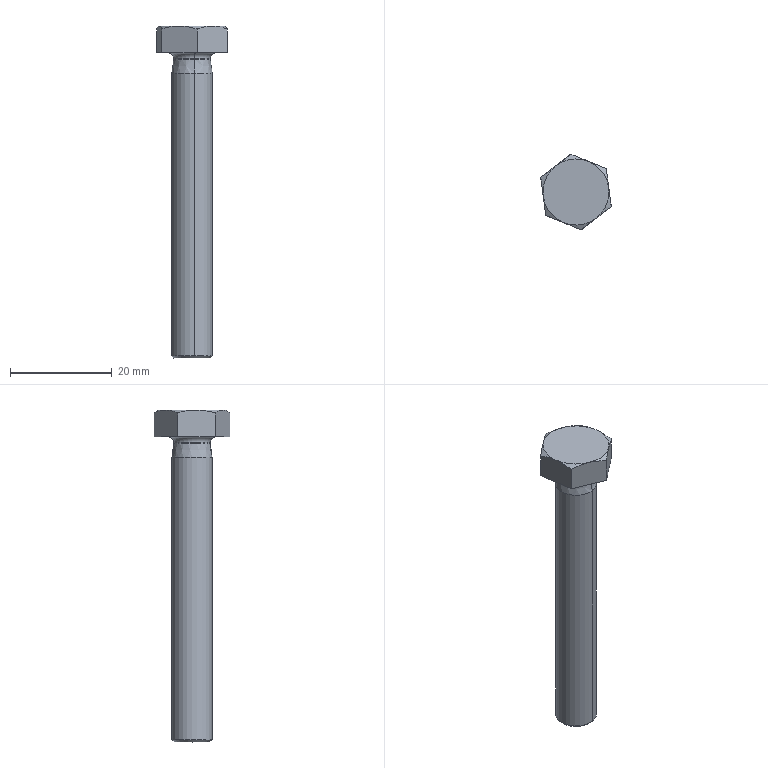Part | STEP file | Chamfer 1-4 | 1 solid | 25 faces | box 13.89 x 14.875 x 65.3 mm | volume 3768 mm3 | cone 10 | plane 9 | torus 4 | cylinder 2 | commonest cylinder face diameters 8 x2
STEP:
#1=CARTESIAN_POINT('',(-881.108,35.613,3046.7));
#2=VERTEX_POINT('',#1);
#3=CARTESIAN_POINT('',(-881.256,36.703,3045.6));
#4=VERTEX_POINT('',#3);
#5=CARTESIAN_POINT('',(-881.108,35.613,3045.6));
#6=DIRECTION('',(-0.991,-0.1342,-0.000000001));
#7=DIRECTION('',(-0.000000001,0.,1.));
#8=AXIS2_PLACEMENT_3D('',#5,#6,#7);
#9=CIRCLE('',#8,1.1);
#10=EDGE_CURVE('',#2,#4,#9,.T.);
#11=ORIENTED_EDGE('',*,*,#10,.T.);
#12=CARTESIAN_POINT('',(-882.221,43.826,3045.6));
#13=VERTEX_POINT('',#12);
#14=CARTESIAN_POINT('',(-881.738,40.264,3045.6));
#15=DIRECTION('',(-0.000000001,0.,1.));
#16=DIRECTION('',(0.1342,-0.991,0.));
#17=AXIS2_PLACEMENT_3D('',#14,#15,#16);
#18=CIRCLE('',#17,3.594);
#19=EDGE_CURVE('',#4,#13,#18,.T.);
#20=ORIENTED_EDGE('',*,*,#19,.T.);
#21=CARTESIAN_POINT('',(-882.368,44.916,3046.7));
#22=VERTEX_POINT('',#21);
#23=CARTESIAN_POINT('',(-882.368,44.916,3045.6));
#24=DIRECTION('',(0.991,0.1342,0.000000001));
#25=DIRECTION('',(0.1342,-0.991,0.));
#26=AXIS2_PLACEMENT_3D('',#23,#24,#25);
#27=CIRCLE('',#26,1.1);
#28=EDGE_CURVE('',#22,#13,#27,.T.);
#29=ORIENTED_EDGE('',*,*,#28,.F.);
#30=CARTESIAN_POINT('',(-881.738,40.264,3046.7));
#31=DIRECTION('',(-0.000000001,0.,1.));
#32=DIRECTION('',(0.1342,-0.991,0.));
#33=AXIS2_PLACEMENT_3D('',#30,#31,#32);
#34=CIRCLE('',#33,4.694);
#35=EDGE_CURVE('',#2,#22,#34,.T.);
#36=ORIENTED_EDGE('',*,*,#35,.F.);
#37=EDGE_LOOP('',(#11,#20,#29,#36));
#38=FACE_OUTER_BOUND('',#37,.T.);
#39=CARTESIAN_POINT('',(-881.738,40.264,3045.6));
#40=DIRECTION('',(-0.000000001,0.,1.));
#41=DIRECTION('',(-0.1342,0.991,0.));
#42=AXIS2_PLACEMENT_3D('',#39,#40,#41);
#43=TOROIDAL_SURFACE('',#42,4.694,1.1);
#44=ADVANCED_FACE('',(#38),#43,.F.);
#45=ORIENTED_EDGE('',*,*,#28,.T.);
#46=CARTESIAN_POINT('',(-881.738,40.264,3045.6));
#47=DIRECTION('',(-0.000000001,0.,1.));
#48=DIRECTION('',(0.1342,-0.991,0.));
#49=AXIS2_PLACEMENT_3D('',#46,#47,#48);
#50=CIRCLE('',#49,3.594);
#51=EDGE_CURVE('',#13,#4,#50,.T.);
#52=ORIENTED_EDGE('',*,*,#51,.T.);
#53=ORIENTED_EDGE('',*,*,#10,.F.);
#54=CARTESIAN_POINT('',(-881.738,40.264,3046.7));
#55=DIRECTION('',(-0.000000001,0.,1.));
#56=DIRECTION('',(0.1342,-0.991,0.));
#57=AXIS2_PLACEMENT_3D('',#54,#55,#56);
#58=CIRCLE('',#57,4.694);
#59=EDGE_CURVE('',#22,#2,#58,.T.);
#60=ORIENTED_EDGE('',*,*,#59,.F.);
#61=EDGE_LOOP('',(#45,#52,#53,#60));
#62=FACE_OUTER_BOUND('',#61,.T.);
#63=CARTESIAN_POINT('',(-881.738,40.264,3045.6));
#64=DIRECTION('',(-0.000000001,0.,1.));
#65=DIRECTION('',(-0.1342,0.991,0.));
#66=AXIS2_PLACEMENT_3D('',#63,#64,#65);
#67=TOROIDAL_SURFACE('',#66,4.694,1.1);
#68=ADVANCED_FACE('',(#62),#67,.F.);
#69=CARTESIAN_POINT('',(-882.215,43.788,2986.7));
#70=VERTEX_POINT('',#69);
#71=CARTESIAN_POINT('',(-881.261,36.741,2986.7));
#72=VERTEX_POINT('',#71);
#73=CARTESIAN_POINT('',(-881.738,40.264,2986.7));
#74=DIRECTION('',(0.000000001,0.,-1.));
#75=DIRECTION('',(0.1342,-0.991,0.));
#76=AXIS2_PLACEMENT_3D('',#73,#74,#75);
#77=CIRCLE('',#76,3.556);
#78=EDGE_CURVE('',#70,#72,#77,.T.);
#79=ORIENTED_EDGE('',*,*,#78,.F.);
#80=CARTESIAN_POINT('',(-882.275,44.228,2987.144));
#81=VERTEX_POINT('',#80);
#82=CARTESIAN_POINT('',(-882.275,44.228,2987.144));
#83=DIRECTION('',(0.09489,-0.7007,-0.7071));
#84=VECTOR('',#83,1000.);
#85=LINE('',#82,#84);
#86=EDGE_CURVE('',#81,#70,#85,.T.);
#87=ORIENTED_EDGE('',*,*,#86,.F.);
#88=CARTESIAN_POINT('',(-881.202,36.3,2987.144));
#89=VERTEX_POINT('',#88);
#90=CARTESIAN_POINT('',(-881.738,40.264,2987.144));
#91=DIRECTION('',(-0.000000001,0.,1.));
#92=DIRECTION('',(0.1342,-0.991,0.));
#93=AXIS2_PLACEMENT_3D('',#90,#91,#92);
#94=CIRCLE('',#93,4.);
#95=EDGE_CURVE('',#89,#81,#94,.T.);
#96=ORIENTED_EDGE('',*,*,#95,.F.);
#97=CARTESIAN_POINT('',(-881.202,36.3,2987.144));
#98=DIRECTION('',(-0.09489,0.7007,-0.7071));
#99=VECTOR('',#98,1000.);
#100=LINE('',#97,#99);
#101=EDGE_CURVE('',#89,#72,#100,.T.);
#102=ORIENTED_EDGE('',*,*,#101,.T.);
#103=EDGE_LOOP('',(#79,#87,#96,#102));
#104=FACE_OUTER_BOUND('',#103,.T.);
#105=CARTESIAN_POINT('',(-881.738,40.264,2987.144));
#106=DIRECTION('',(-0.000000001,0.,1.));
#107=DIRECTION('',(-0.1342,0.991,0.));
#108=AXIS2_PLACEMENT_3D('',#105,#106,#107);
#109=CONICAL_SURFACE('',#108,4.,0.7854);
#110=ADVANCED_FACE('',(#104),#109,.T.);
#111=ORIENTED_EDGE('',*,*,#51,.F.);
#112=CARTESIAN_POINT('',(-882.222,43.837,3045.443));
#113=VERTEX_POINT('',#112);
#114=CARTESIAN_POINT('',(-882.368,44.916,3045.6));
#115=DIRECTION('',(-0.991,-0.1342,-0.000000001));
#116=DIRECTION('',(0.1342,-0.991,0.));
#117=AXIS2_PLACEMENT_3D('',#114,#115,#116);
#118=CIRCLE('',#117,1.1);
#119=EDGE_CURVE('',#113,#13,#118,.T.);
#120=ORIENTED_EDGE('',*,*,#119,.F.);
#121=CARTESIAN_POINT('',(-881.254,36.692,3045.443));
#122=VERTEX_POINT('',#121);
#123=CARTESIAN_POINT('',(-881.738,40.264,3045.443));
#124=DIRECTION('',(-0.000000001,0.,1.));
#125=DIRECTION('',(0.1342,-0.991,0.));
#126=AXIS2_PLACEMENT_3D('',#123,#124,#125);
#127=CIRCLE('',#126,3.605);
#128=EDGE_CURVE('',#113,#122,#127,.T.);
#129=ORIENTED_EDGE('',*,*,#128,.T.);
#130=CARTESIAN_POINT('',(-881.108,35.613,3045.6));
#131=DIRECTION('',(0.991,0.1342,0.000000001));
#132=DIRECTION('',(-0.000000001,0.,1.));
#133=AXIS2_PLACEMENT_3D('',#130,#131,#132);
#134=CIRCLE('',#133,1.1);
#135=EDGE_CURVE('',#122,#4,#134,.T.);
#136=ORIENTED_EDGE('',*,*,#135,.T.);
#137=EDGE_LOOP('',(#111,#120,#129,#136));
#138=FACE_OUTER_BOUND('',#137,.T.);
#139=CARTESIAN_POINT('',(-881.738,40.264,3045.6));
#140=DIRECTION('',(-0.000000001,0.,1.));
#141=DIRECTION('',(-0.1342,0.991,0.));
#142=AXIS2_PLACEMENT_3D('',#139,#140,#141);
#143=TOROIDAL_SURFACE('',#142,4.694,1.1);
#144=ADVANCED_FACE('',(#138),#143,.F.);
#145=ORIENTED_EDGE('',*,*,#95,.T.);
#146=CARTESIAN_POINT('',(-882.275,44.228,3042.7));
#147=VERTEX_POINT('',#146);
#148=CARTESIAN_POINT('',(-882.275,44.228,3046.7));
#149=DIRECTION('',(0.000000001,0.,-1.));
#150=VECTOR('',#149,1000.);
#151=LINE('',#148,#150);
#152=EDGE_CURVE('',#147,#81,#151,.T.);
#153=ORIENTED_EDGE('',*,*,#152,.F.);
#154=CARTESIAN_POINT('',(-881.202,36.3,3042.7));
#155=VERTEX_POINT('',#154);
#156=CARTESIAN_POINT('',(-881.738,40.264,3042.7));
#157=DIRECTION('',(-0.000000001,0.,1.));
#158=DIRECTION('',(0.1342,-0.991,0.));
#159=AXIS2_PLACEMENT_3D('',#156,#157,#158);
#160=CIRCLE('',#159,4.);
#161=EDGE_CURVE('',#155,#147,#160,.T.);
#162=ORIENTED_EDGE('',*,*,#161,.F.);
#163=CARTESIAN_POINT('',(-881.202,36.3,3046.7));
#164=DIRECTION('',(0.000000001,0.,-1.));
#165=VECTOR('',#164,1000.);
#166=LINE('',#163,#165);
#167=EDGE_CURVE('',#155,#89,#166,.T.);
#168=ORIENTED_EDGE('',*,*,#167,.T.);
#169=EDGE_LOOP('',(#145,#153,#162,#168));
#170=FACE_OUTER_BOUND('',#169,.T.);
#171=CARTESIAN_POINT('',(-881.738,40.264,3046.7));
#172=DIRECTION('',(-0.000000001,0.,1.));
#173=DIRECTION('',(-0.1342,0.991,0.));
#174=AXIS2_PLACEMENT_3D('',#171,#172,#173);
#175=CYLINDRICAL_SURFACE('',#174,4.);
#176=ADVANCED_FACE('',(#170),#175,.T.);
#177=CARTESIAN_POINT('',(-881.738,40.264,3045.443));
#178=DIRECTION('',(-0.000000001,0.,1.));
#179=DIRECTION('',(0.1342,-0.991,0.));
#180=AXIS2_PLACEMENT_3D('',#177,#178,#179);
#181=CIRCLE('',#180,3.605);
#182=EDGE_CURVE('',#122,#113,#181,.T.);
#183=ORIENTED_EDGE('',*,*,#182,.F.);
#184=CARTESIAN_POINT('',(-881.202,36.3,3042.7));
#185=DIRECTION('',(0.01911,-0.1411,-0.9898));
#186=VECTOR('',#185,1000.);
#187=LINE('',#184,#186);
#188=EDGE_CURVE('',#122,#155,#187,.T.);
#189=ORIENTED_EDGE('',*,*,#188,.T.);
#190=ORIENTED_EDGE('',*,*,#161,.T.);
#191=CARTESIAN_POINT('',(-882.275,44.228,3042.7));
#192=DIRECTION('',(-0.01911,0.1411,-0.9898));
#193=VECTOR('',#192,1000.);
#194=LINE('',#191,#193);
#195=EDGE_CURVE('',#113,#147,#194,.T.);
#196=ORIENTED_EDGE('',*,*,#195,.F.);
#197=EDGE_LOOP('',(#183,#189,#190,#196));
#198=FACE_OUTER_BOUND('',#197,.T.);
#199=CARTESIAN_POINT('',(-881.738,40.264,3042.7));
#200=DIRECTION('',(0.000000001,0.,-1.));
#201=DIRECTION('',(0.1342,-0.991,0.));
#202=AXIS2_PLACEMENT_3D('',#199,#200,#201);
#203=CONICAL_SURFACE('',#202,4.,0.1429);
#204=ADVANCED_FACE('',(#198),#203,.T.);
#205=CARTESIAN_POINT('',(-887.676,35.673,3046.7));
#206=VERTEX_POINT('',#205);
#207=CARTESIAN_POINT('',(-888.683,43.111,3046.7));
#208=VERTEX_POINT('',#207);
#209=CARTESIAN_POINT('',(-887.676,35.673,3046.7));
#210=DIRECTION('',(-0.1342,0.991,0.));
#211=VECTOR('',#210,1000.);
#212=LINE('',#209,#211);
#213=EDGE_CURVE('',#206,#208,#212,.T.);
#214=ORIENTED_EDGE('',*,*,#213,.T.);
#215=CARTESIAN_POINT('',(-882.745,47.702,3046.7));
#216=VERTEX_POINT('',#215);
#217=CARTESIAN_POINT('',(-888.683,43.111,3046.7));
#218=DIRECTION('',(0.7911,0.6117,0.));
#219=VECTOR('',#218,1000.);
#220=LINE('',#217,#219);
#221=EDGE_CURVE('',#208,#216,#220,.T.);
#222=ORIENTED_EDGE('',*,*,#221,.T.);
#223=CARTESIAN_POINT('',(-875.801,44.855,3046.7));
#224=VERTEX_POINT('',#223);
#225=CARTESIAN_POINT('',(-882.745,47.702,3046.7));
#226=DIRECTION('',(0.9253,-0.3793,0.000000001));
#227=VECTOR('',#226,1000.);
#228=LINE('',#225,#227);
#229=EDGE_CURVE('',#216,#224,#228,.T.);
#230=ORIENTED_EDGE('',*,*,#229,.T.);
#231=CARTESIAN_POINT('',(-874.793,37.418,3046.7));
#232=VERTEX_POINT('',#231);
#233=CARTESIAN_POINT('',(-875.801,44.855,3046.7));
#234=DIRECTION('',(0.1342,-0.991,0.));
#235=VECTOR('',#234,1000.);
#236=LINE('',#233,#235);
#237=EDGE_CURVE('',#224,#232,#236,.T.);
#238=ORIENTED_EDGE('',*,*,#237,.T.);
#239=CARTESIAN_POINT('',(-880.731,32.827,3046.7));
#240=VERTEX_POINT('',#239);
#241=CARTESIAN_POINT('',(-874.793,37.418,3046.7));
#242=DIRECTION('',(-0.7911,-0.6117,0.));
#243=VECTOR('',#242,1000.);
#244=LINE('',#241,#243);
#245=EDGE_CURVE('',#232,#240,#244,.T.);
#246=ORIENTED_EDGE('',*,*,#245,.T.);
#247=CARTESIAN_POINT('',(-880.731,32.827,3046.7));
#248=DIRECTION('',(-0.9253,0.3793,-0.000000001));
#249=VECTOR('',#248,1000.);
#250=LINE('',#247,#249);
#251=EDGE_CURVE('',#240,#206,#250,.T.);
#252=ORIENTED_EDGE('',*,*,#251,.T.);
#253=EDGE_LOOP('',(#214,#222,#230,#238,#246,#252));
#254=FACE_OUTER_BOUND('',#253,.T.);
#255=ORIENTED_EDGE('',*,*,#35,.T.);
#256=ORIENTED_EDGE('',*,*,#59,.T.);
#257=EDGE_LOOP('',(#255,#256));
#258=FACE_BOUND('',#257,.T.);
#259=CARTESIAN_POINT('',(-888.683,43.111,3046.7));
#260=DIRECTION('',(0.000000001,0.,-1.));
#261=DIRECTION('',(0.991,0.1342,0.000000001));
#262=AXIS2_PLACEMENT_3D('',#259,#260,#261);
#263=PLANE('',#262);
#264=ADVANCED_FACE('',(#254,#258),#263,.T.);
#265=CARTESIAN_POINT('',(-888.683,43.111,3051.419));
#266=VERTEX_POINT('',#265);
#267=CARTESIAN_POINT('',(-888.179,39.392,3052.));
#268=VERTEX_POINT('',#267);
#269=CARTESIAN_POINT('',(-888.683,43.111,3051.419));
#270=CARTESIAN_POINT('',(-888.519,41.896,3051.773));
#271=CARTESIAN_POINT('',(-888.351,40.661,3052.));
#272=CARTESIAN_POINT('',(-888.179,39.392,3052.));
#273=B_SPLINE_CURVE_WITH_KNOTS('',3,(#269,#270,#271,#272),.UNSPECIFIED.,.F.,.F.,(4,4),(0.,0.003797),.UNSPECIFIED.);
#274=EDGE_CURVE('',#266,#268,#273,.T.);
#275=ORIENTED_EDGE('',*,*,#274,.F.);
#276=CARTESIAN_POINT('',(-888.683,43.111,3046.7));
#277=DIRECTION('',(-0.000000001,0.,1.));
#278=VECTOR('',#277,1000.);
#279=LINE('',#276,#278);
#280=EDGE_CURVE('',#208,#266,#279,.T.);
#281=ORIENTED_EDGE('',*,*,#280,.F.);
#282=ORIENTED_EDGE('',*,*,#213,.F.);
#283=CARTESIAN_POINT('',(-887.676,35.673,3051.419));
#284=VERTEX_POINT('',#283);
#285=CARTESIAN_POINT('',(-887.676,35.673,3046.7));
#286=DIRECTION('',(-0.000000001,0.,1.));
#287=VECTOR('',#286,1000.);
#288=LINE('',#285,#287);
#289=EDGE_CURVE('',#206,#284,#288,.T.);
#290=ORIENTED_EDGE('',*,*,#289,.T.);
#291=CARTESIAN_POINT('',(-888.179,39.392,3052.));
#292=CARTESIAN_POINT('',(-888.008,38.123,3052.));
#293=CARTESIAN_POINT('',(-887.84,36.888,3051.773));
#294=CARTESIAN_POINT('',(-887.676,35.673,3051.419));
#295=B_SPLINE_CURVE_WITH_KNOTS('',3,(#291,#292,#293,#294),.UNSPECIFIED.,.F.,.F.,(4,4),(0.,0.003797),.UNSPECIFIED.);
#296=EDGE_CURVE('',#268,#284,#295,.T.);
#297=ORIENTED_EDGE('',*,*,#296,.F.);
#298=EDGE_LOOP('',(#275,#281,#282,#290,#297));
#299=FACE_OUTER_BOUND('',#298,.T.);
#300=CARTESIAN_POINT('',(-887.676,35.673,3046.7));
#301=DIRECTION('',(0.991,0.1342,0.000000001));
#302=DIRECTION('',(-0.1342,0.991,0.));
#303=AXIS2_PLACEMENT_3D('',#300,#301,#302);
#304=PLANE('',#303);
#305=ADVANCED_FACE('',(#299),#304,.F.);
#306=CARTESIAN_POINT('',(-882.745,47.702,3051.419));
#307=VERTEX_POINT('',#306);
#308=CARTESIAN_POINT('',(-885.714,45.406,3052.));
#309=VERTEX_POINT('',#308);
#310=CARTESIAN_POINT('',(-882.745,47.702,3051.419));
#311=CARTESIAN_POINT('',(-883.715,46.952,3051.773));
#312=CARTESIAN_POINT('',(-884.701,46.19,3052.));
#313=CARTESIAN_POINT('',(-885.714,45.406,3052.));
#314=B_SPLINE_CURVE_WITH_KNOTS('',3,(#310,#311,#312,#313),.UNSPECIFIED.,.F.,.F.,(4,4),(0.,0.003797),.UNSPECIFIED.);
#315=EDGE_CURVE('',#307,#309,#314,.T.);
#316=ORIENTED_EDGE('',*,*,#315,.F.);
#317=CARTESIAN_POINT('',(-882.745,47.702,3046.7));
#318=DIRECTION('',(-0.000000001,0.,1.));
#319=VECTOR('',#318,1000.);
#320=LINE('',#317,#319);
#321=EDGE_CURVE('',#216,#307,#320,.T.);
#322=ORIENTED_EDGE('',*,*,#321,.F.);
#323=ORIENTED_EDGE('',*,*,#221,.F.);
#324=ORIENTED_EDGE('',*,*,#280,.T.);
#325=CARTESIAN_POINT('',(-885.714,45.406,3052.));
#326=CARTESIAN_POINT('',(-886.728,44.623,3052.));
#327=CARTESIAN_POINT('',(-887.713,43.861,3051.773));
#328=CARTESIAN_POINT('',(-888.683,43.111,3051.419));
#329=B_SPLINE_CURVE_WITH_KNOTS('',3,(#325,#326,#327,#328),.UNSPECIFIED.,.F.,.F.,(4,4),(0.,0.003797),.UNSPECIFIED.);
#330=EDGE_CURVE('',#309,#266,#329,.T.);
#331=ORIENTED_EDGE('',*,*,#330,.F.);
#332=EDGE_LOOP('',(#316,#322,#323,#324,#331));
#333=FACE_OUTER_BOUND('',#332,.T.);
#334=CARTESIAN_POINT('',(-888.683,43.111,3046.7));
#335=DIRECTION('',(0.6117,-0.7911,0.));
#336=DIRECTION('',(0.7911,0.6117,0.));
#337=AXIS2_PLACEMENT_3D('',#334,#335,#336);
#338=PLANE('',#337);
#339=ADVANCED_FACE('',(#333),#338,.F.);
#340=CARTESIAN_POINT('',(-875.801,44.855,3051.419));
#341=VERTEX_POINT('',#340);
#342=CARTESIAN_POINT('',(-879.273,46.279,3052.));
#343=VERTEX_POINT('',#342);
#344=CARTESIAN_POINT('',(-875.801,44.855,3051.419));
#345=CARTESIAN_POINT('',(-876.935,45.32,3051.773));
#346=CARTESIAN_POINT('',(-878.088,45.793,3052.));
#347=CARTESIAN_POINT('',(-879.273,46.279,3052.));
#348=B_SPLINE_CURVE_WITH_KNOTS('',3,(#344,#345,#346,#347),.UNSPECIFIED.,.F.,.F.,(4,4),(0.,0.003797),.UNSPECIFIED.);
#349=EDGE_CURVE('',#341,#343,#348,.T.);
#350=ORIENTED_EDGE('',*,*,#349,.F.);
#351=CARTESIAN_POINT('',(-875.801,44.855,3046.7));
#352=DIRECTION('',(-0.000000001,0.,1.));
#353=VECTOR('',#352,1000.);
#354=LINE('',#351,#353);
#355=EDGE_CURVE('',#224,#341,#354,.T.);
#356=ORIENTED_EDGE('',*,*,#355,.F.);
#357=ORIENTED_EDGE('',*,*,#229,.F.);
#358=ORIENTED_EDGE('',*,*,#321,.T.);
#359=CARTESIAN_POINT('',(-879.273,46.279,3052.));
#360=CARTESIAN_POINT('',(-880.458,46.764,3052.));
#361=CARTESIAN_POINT('',(-881.611,47.237,3051.773));
#362=CARTESIAN_POINT('',(-882.745,47.702,3051.419));
#363=B_SPLINE_CURVE_WITH_KNOTS('',3,(#359,#360,#361,#362),.UNSPECIFIED.,.F.,.F.,(4,4),(0.,0.003797),.UNSPECIFIED.);
#364=EDGE_CURVE('',#343,#307,#363,.T.);
#365=ORIENTED_EDGE('',*,*,#364,.F.);
#366=EDGE_LOOP('',(#350,#356,#357,#358,#365));
#367=FACE_OUTER_BOUND('',#366,.T.);
#368=CARTESIAN_POINT('',(-882.745,47.702,3046.7));
#369=DIRECTION('',(-0.3793,-0.9253,0.));
#370=DIRECTION('',(0.9253,-0.3793,0.000000001));
#371=AXIS2_PLACEMENT_3D('',#368,#369,#370);
#372=PLANE('',#371);
#373=ADVANCED_FACE('',(#367),#372,.F.);
#374=CARTESIAN_POINT('',(-874.793,37.418,3051.419));
#375=VERTEX_POINT('',#374);
#376=CARTESIAN_POINT('',(-875.297,41.137,3052.));
#377=VERTEX_POINT('',#376);
#378=CARTESIAN_POINT('',(-874.793,37.418,3051.419));
#379=CARTESIAN_POINT('',(-874.958,38.633,3051.773));
#380=CARTESIAN_POINT('',(-875.125,39.867,3052.));
#381=CARTESIAN_POINT('',(-875.297,41.137,3052.));
#382=B_SPLINE_CURVE_WITH_KNOTS('',3,(#378,#379,#380,#381),.UNSPECIFIED.,.F.,.F.,(4,4),(0.,0.003797),.UNSPECIFIED.);
#383=EDGE_CURVE('',#375,#377,#382,.T.);
#384=ORIENTED_EDGE('',*,*,#383,.F.);
#385=CARTESIAN_POINT('',(-874.793,37.418,3046.7));
#386=DIRECTION('',(-0.000000001,0.,1.));
#387=VECTOR('',#386,1000.);
#388=LINE('',#385,#387);
#389=EDGE_CURVE('',#232,#375,#388,.T.);
#390=ORIENTED_EDGE('',*,*,#389,.F.);
#391=ORIENTED_EDGE('',*,*,#237,.F.);
#392=ORIENTED_EDGE('',*,*,#355,.T.);
#393=CARTESIAN_POINT('',(-875.297,41.137,3052.));
#394=CARTESIAN_POINT('',(-875.469,42.406,3052.));
#395=CARTESIAN_POINT('',(-875.636,43.64,3051.773));
#396=CARTESIAN_POINT('',(-875.801,44.855,3051.419));
#397=B_SPLINE_CURVE_WITH_KNOTS('',3,(#393,#394,#395,#396),.UNSPECIFIED.,.F.,.F.,(4,4),(0.,0.003797),.UNSPECIFIED.);
#398=EDGE_CURVE('',#377,#341,#397,.T.);
#399=ORIENTED_EDGE('',*,*,#398,.F.);
#400=EDGE_LOOP('',(#384,#390,#391,#392,#399));
#401=FACE_OUTER_BOUND('',#400,.T.);
#402=CARTESIAN_POINT('',(-875.801,44.855,3046.7));
#403=DIRECTION('',(-0.991,-0.1342,-0.000000001));
#404=DIRECTION('',(0.000000001,0.,-1.));
#405=AXIS2_PLACEMENT_3D('',#402,#403,#404);
#406=PLANE('',#405);
#407=ADVANCED_FACE('',(#401),#406,.F.);
#408=CARTESIAN_POINT('',(-880.731,32.827,3051.419));
#409=VERTEX_POINT('',#408);
#410=CARTESIAN_POINT('',(-877.762,35.122,3052.));
#411=VERTEX_POINT('',#410);
#412=CARTESIAN_POINT('',(-880.731,32.827,3051.419));
#413=CARTESIAN_POINT('',(-879.761,33.577,3051.773));
#414=CARTESIAN_POINT('',(-878.776,34.339,3052.));
#415=CARTESIAN_POINT('',(-877.762,35.122,3052.));
#416=B_SPLINE_CURVE_WITH_KNOTS('',3,(#412,#413,#414,#415),.UNSPECIFIED.,.F.,.F.,(4,4),(0.,0.003797),.UNSPECIFIED.);
#417=EDGE_CURVE('',#409,#411,#416,.T.);
#418=ORIENTED_EDGE('',*,*,#417,.F.);
#419=CARTESIAN_POINT('',(-880.731,32.827,3046.7));
#420=DIRECTION('',(-0.000000001,0.,1.));
#421=VECTOR('',#420,1000.);
#422=LINE('',#419,#421);
#423=EDGE_CURVE('',#240,#409,#422,.T.);
#424=ORIENTED_EDGE('',*,*,#423,.F.);
#425=ORIENTED_EDGE('',*,*,#245,.F.);
#426=ORIENTED_EDGE('',*,*,#389,.T.);
#427=CARTESIAN_POINT('',(-877.762,35.122,3052.));
#428=CARTESIAN_POINT('',(-876.749,35.906,3052.));
#429=CARTESIAN_POINT('',(-875.763,36.668,3051.773));
#430=CARTESIAN_POINT('',(-874.793,37.418,3051.419));
#431=B_SPLINE_CURVE_WITH_KNOTS('',3,(#427,#428,#429,#430),.UNSPECIFIED.,.F.,.F.,(4,4),(0.,0.003797),.UNSPECIFIED.);
#432=EDGE_CURVE('',#411,#375,#431,.T.);
#433=ORIENTED_EDGE('',*,*,#432,.F.);
#434=EDGE_LOOP('',(#418,#424,#425,#426,#433));
#435=FACE_OUTER_BOUND('',#434,.T.);
#436=CARTESIAN_POINT('',(-874.793,37.418,3046.7));
#437=DIRECTION('',(-0.6117,0.7911,0.));
#438=DIRECTION('',(-0.7911,-0.6117,0.));
#439=AXIS2_PLACEMENT_3D('',#436,#437,#438);
#440=PLANE('',#439);
#441=ADVANCED_FACE('',(#435),#440,.F.);
#442=CARTESIAN_POINT('',(-884.203,34.25,3052.));
#443=VERTEX_POINT('',#442);
#444=CARTESIAN_POINT('',(-887.676,35.673,3051.419));
#445=CARTESIAN_POINT('',(-886.541,35.208,3051.773));
#446=CARTESIAN_POINT('',(-885.389,34.736,3052.));
#447=CARTESIAN_POINT('',(-884.203,34.25,3052.));
#448=B_SPLINE_CURVE_WITH_KNOTS('',3,(#444,#445,#446,#447),.UNSPECIFIED.,.F.,.F.,(4,4),(0.,0.003797),.UNSPECIFIED.);
#449=EDGE_CURVE('',#284,#443,#448,.T.);
#450=ORIENTED_EDGE('',*,*,#449,.F.);
#451=ORIENTED_EDGE('',*,*,#289,.F.);
#452=ORIENTED_EDGE('',*,*,#251,.F.);
#453=ORIENTED_EDGE('',*,*,#423,.T.);
#454=CARTESIAN_POINT('',(-884.203,34.25,3052.));
#455=CARTESIAN_POINT('',(-883.018,33.764,3052.));
#456=CARTESIAN_POINT('',(-881.866,33.292,3051.773));
#457=CARTESIAN_POINT('',(-880.731,32.827,3051.419));
#458=B_SPLINE_CURVE_WITH_KNOTS('',3,(#454,#455,#456,#457),.UNSPECIFIED.,.F.,.F.,(4,4),(0.,0.003797),.UNSPECIFIED.);
#459=EDGE_CURVE('',#443,#409,#458,.T.);
#460=ORIENTED_EDGE('',*,*,#459,.F.);
#461=EDGE_LOOP('',(#450,#451,#452,#453,#460));
#462=FACE_OUTER_BOUND('',#461,.T.);
#463=CARTESIAN_POINT('',(-880.731,32.827,3046.7));
#464=DIRECTION('',(0.3793,0.9253,0.));
#465=DIRECTION('',(-0.9253,0.3793,-0.000000001));
#466=AXIS2_PLACEMENT_3D('',#463,#464,#465);
#467=PLANE('',#466);
#468=ADVANCED_FACE('',(#462),#467,.F.);
#469=ORIENTED_EDGE('',*,*,#296,.T.);
#470=ORIENTED_EDGE('',*,*,#449,.T.);
#471=CARTESIAN_POINT('',(-881.738,40.264,3052.));
#472=DIRECTION('',(0.000000001,0.,-1.));
#473=DIRECTION('',(-0.991,-0.1342,-0.000000001));
#474=AXIS2_PLACEMENT_3D('',#471,#472,#473);
#475=CIRCLE('',#474,6.5);
#476=EDGE_CURVE('',#443,#268,#475,.T.);
#477=ORIENTED_EDGE('',*,*,#476,.T.);
#478=EDGE_LOOP('',(#469,#470,#477));
#479=FACE_OUTER_BOUND('',#478,.T.);
#480=CARTESIAN_POINT('',(-881.738,40.264,3052.));
#481=DIRECTION('',(0.000000001,0.,-1.));
#482=DIRECTION('',(-0.991,-0.1342,-0.000000001));
#483=AXIS2_PLACEMENT_3D('',#480,#481,#482);
#484=CONICAL_SURFACE('',#483,6.5,1.047);
#485=ADVANCED_FACE('',(#479),#484,.T.);
#486=ORIENTED_EDGE('',*,*,#417,.T.);
#487=CARTESIAN_POINT('',(-881.738,40.264,3052.));
#488=DIRECTION('',(0.000000001,0.,-1.));
#489=DIRECTION('',(-0.991,-0.1342,-0.000000001));
#490=AXIS2_PLACEMENT_3D('',#487,#488,#489);
#491=CIRCLE('',#490,6.5);
#492=EDGE_CURVE('',#411,#443,#491,.T.);
#493=ORIENTED_EDGE('',*,*,#492,.T.);
#494=ORIENTED_EDGE('',*,*,#459,.T.);
#495=EDGE_LOOP('',(#486,#493,#494));
#496=FACE_OUTER_BOUND('',#495,.T.);
#497=CARTESIAN_POINT('',(-881.738,40.264,3052.));
#498=DIRECTION('',(0.000000001,0.,-1.));
#499=DIRECTION('',(-0.991,-0.1342,-0.000000001));
#500=AXIS2_PLACEMENT_3D('',#497,#498,#499);
#501=CONICAL_SURFACE('',#500,6.5,1.047);
#502=ADVANCED_FACE('',(#496),#501,.T.);
#503=ORIENTED_EDGE('',*,*,#383,.T.);
#504=CARTESIAN_POINT('',(-881.738,40.264,3052.));
#505=DIRECTION('',(0.000000001,0.,-1.));
#506=DIRECTION('',(-0.991,-0.1342,-0.000000001));
#507=AXIS2_PLACEMENT_3D('',#504,#505,#506);
#508=CIRCLE('',#507,6.5);
#509=EDGE_CURVE('',#377,#411,#508,.T.);
#510=ORIENTED_EDGE('',*,*,#509,.T.);
#511=ORIENTED_EDGE('',*,*,#432,.T.);
#512=EDGE_LOOP('',(#503,#510,#511));
#513=FACE_OUTER_BOUND('',#512,.T.);
#514=CARTESIAN_POINT('',(-881.738,40.264,3052.));
#515=DIRECTION('',(0.000000001,0.,-1.));
#516=DIRECTION('',(-0.991,-0.1342,-0.000000001));
#517=AXIS2_PLACEMENT_3D('',#514,#515,#516);
#518=CONICAL_SURFACE('',#517,6.5,1.047);
#519=ADVANCED_FACE('',(#513),#518,.T.);
#520=ORIENTED_EDGE('',*,*,#349,.T.);
#521=CARTESIAN_POINT('',(-881.738,40.264,3052.));
#522=DIRECTION('',(-0.000000001,0.,1.));
#523=DIRECTION('',(0.991,0.1342,0.000000001));
#524=AXIS2_PLACEMENT_3D('',#521,#522,#523);
#525=CIRCLE('',#524,6.5);
#526=EDGE_CURVE('',#377,#343,#525,.T.);
#527=ORIENTED_EDGE('',*,*,#526,.F.);
#528=ORIENTED_EDGE('',*,*,#398,.T.);
#529=EDGE_LOOP('',(#520,#527,#528));
#530=FACE_OUTER_BOUND('',#529,.T.);
#531=CARTESIAN_POINT('',(-881.738,40.264,3052.));
#532=DIRECTION('',(0.000000001,0.,-1.));
#533=DIRECTION('',(-0.991,-0.1342,-0.000000001));
#534=AXIS2_PLACEMENT_3D('',#531,#532,#533);
#535=CONICAL_SURFACE('',#534,6.5,1.047);
#536=ADVANCED_FACE('',(#530),#535,.T.);
#537=ORIENTED_EDGE('',*,*,#364,.T.);
#538=ORIENTED_EDGE('',*,*,#315,.T.);
#539=CARTESIAN_POINT('',(-881.738,40.264,3052.));
#540=DIRECTION('',(0.000000001,0.,-1.));
#541=DIRECTION('',(-0.991,-0.1342,-0.000000001));
#542=AXIS2_PLACEMENT_3D('',#539,#540,#541);
#543=CIRCLE('',#542,6.5);
#544=EDGE_CURVE('',#309,#343,#543,.T.);
#545=ORIENTED_EDGE('',*,*,#544,.T.);
#546=EDGE_LOOP('',(#537,#538,#545));
#547=FACE_OUTER_BOUND('',#546,.T.);
#548=CARTESIAN_POINT('',(-881.738,40.264,3052.));
#549=DIRECTION('',(0.000000001,0.,-1.));
#550=DIRECTION('',(-0.991,-0.1342,-0.000000001));
#551=AXIS2_PLACEMENT_3D('',#548,#549,#550);
#552=CONICAL_SURFACE('',#551,6.5,1.047);
#553=ADVANCED_FACE('',(#547),#552,.T.);
#554=ORIENTED_EDGE('',*,*,#330,.T.);
#555=ORIENTED_EDGE('',*,*,#274,.T.);
#556=CARTESIAN_POINT('',(-881.738,40.264,3052.));
#557=DIRECTION('',(0.000000001,0.,-1.));
#558=DIRECTION('',(-0.991,-0.1342,-0.000000001));
#559=AXIS2_PLACEMENT_3D('',#556,#557,#558);
#560=CIRCLE('',#559,6.5);
#561=EDGE_CURVE('',#268,#309,#560,.T.);
#562=ORIENTED_EDGE('',*,*,#561,.T.);
#563=EDGE_LOOP('',(#554,#555,#562));
#564=FACE_OUTER_BOUND('',#563,.T.);
#565=CARTESIAN_POINT('',(-881.738,40.264,3052.));
#566=DIRECTION('',(0.000000001,0.,-1.));
#567=DIRECTION('',(-0.991,-0.1342,-0.000000001));
#568=AXIS2_PLACEMENT_3D('',#565,#566,#567);
#569=CONICAL_SURFACE('',#568,6.5,1.047);
#570=ADVANCED_FACE('',(#564),#569,.T.);
#571=ORIENTED_EDGE('',*,*,#561,.F.);
#572=ORIENTED_EDGE('',*,*,#476,.F.);
#573=ORIENTED_EDGE('',*,*,#492,.F.);
#574=ORIENTED_EDGE('',*,*,#509,.F.);
#575=ORIENTED_EDGE('',*,*,#526,.T.);
#576=ORIENTED_EDGE('',*,*,#544,.F.);
#577=EDGE_LOOP('',(#571,#572,#573,#574,#575,#576));
#578=FACE_OUTER_BOUND('',#577,.T.);
#579=CARTESIAN_POINT('',(-888.683,43.111,3052.));
#580=DIRECTION('',(0.000000001,0.,-1.));
#581=DIRECTION('',(0.991,0.1342,0.000000001));
#582=AXIS2_PLACEMENT_3D('',#579,#580,#581);
#583=PLANE('',#582);
#584=ADVANCED_FACE('',(#578),#583,.F.);
#585=ORIENTED_EDGE('',*,*,#188,.F.);
#586=ORIENTED_EDGE('',*,*,#128,.F.);
#587=ORIENTED_EDGE('',*,*,#195,.T.);
#588=CARTESIAN_POINT('',(-881.738,40.264,3042.7));
#589=DIRECTION('',(-0.000000001,0.,1.));
#590=DIRECTION('',(0.1342,-0.991,0.));
#591=AXIS2_PLACEMENT_3D('',#588,#589,#590);
#592=CIRCLE('',#591,4.);
#593=EDGE_CURVE('',#147,#155,#592,.T.);
#594=ORIENTED_EDGE('',*,*,#593,.T.);
#595=EDGE_LOOP('',(#585,#586,#587,#594));
#596=FACE_OUTER_BOUND('',#595,.T.);
#597=CARTESIAN_POINT('',(-881.738,40.264,3042.7));
#598=DIRECTION('',(0.000000001,0.,-1.));
#599=DIRECTION('',(0.1342,-0.991,0.));
#600=AXIS2_PLACEMENT_3D('',#597,#598,#599);
#601=CONICAL_SURFACE('',#600,4.,0.1429);
#602=ADVANCED_FACE('',(#596),#601,.T.);
#603=ORIENTED_EDGE('',*,*,#152,.T.);
#604=CARTESIAN_POINT('',(-881.738,40.264,2987.144));
#605=DIRECTION('',(-0.000000001,0.,1.));
#606=DIRECTION('',(0.1342,-0.991,0.));
#607=AXIS2_PLACEMENT_3D('',#604,#605,#606);
#608=CIRCLE('',#607,4.);
#609=EDGE_CURVE('',#81,#89,#608,.T.);
#610=ORIENTED_EDGE('',*,*,#609,.T.);
#611=ORIENTED_EDGE('',*,*,#167,.F.);
#612=ORIENTED_EDGE('',*,*,#593,.F.);
#613=EDGE_LOOP('',(#603,#610,#611,#612));
#614=FACE_OUTER_BOUND('',#613,.T.);
#615=CARTESIAN_POINT('',(-881.738,40.264,3046.7));
#616=DIRECTION('',(-0.000000001,0.,1.));
#617=DIRECTION('',(-0.1342,0.991,0.));
#618=AXIS2_PLACEMENT_3D('',#615,#616,#617);
#619=CYLINDRICAL_SURFACE('',#618,4.);
#620=ADVANCED_FACE('',(#614),#619,.T.);
#621=CARTESIAN_POINT('',(-881.738,40.264,2986.7));
#622=DIRECTION('',(0.000000001,0.,-1.));
#623=DIRECTION('',(0.1342,-0.991,0.));
#624=AXIS2_PLACEMENT_3D('',#621,#622,#623);
#625=CIRCLE('',#624,3.556);
#626=EDGE_CURVE('',#72,#70,#625,.T.);
#627=ORIENTED_EDGE('',*,*,#626,.T.);
#628=ORIENTED_EDGE('',*,*,#78,.T.);
#629=EDGE_LOOP('',(#627,#628));
#630=FACE_OUTER_BOUND('',#629,.T.);
#631=CARTESIAN_POINT('',(-882.275,44.228,2986.7));
#632=DIRECTION('',(-0.000000001,0.,1.));
#633=DIRECTION('',(-0.1342,0.991,0.));
#634=AXIS2_PLACEMENT_3D('',#631,#632,#633);
#635=PLANE('',#634);
#636=ADVANCED_FACE('',(#630),#635,.F.);
#637=ORIENTED_EDGE('',*,*,#19,.F.);
#638=ORIENTED_EDGE('',*,*,#135,.F.);
#639=ORIENTED_EDGE('',*,*,#182,.T.);
#640=ORIENTED_EDGE('',*,*,#119,.T.);
#641=EDGE_LOOP('',(#637,#638,#639,#640));
#642=FACE_OUTER_BOUND('',#641,.T.);
#643=CARTESIAN_POINT('',(-881.738,40.264,3045.6));
#644=DIRECTION('',(-0.000000001,0.,1.));
#645=DIRECTION('',(-0.1342,0.991,0.));
#646=AXIS2_PLACEMENT_3D('',#643,#644,#645);
#647=TOROIDAL_SURFACE('',#646,4.694,1.1);
#648=ADVANCED_FACE('',(#642),#647,.F.);
#649=ORIENTED_EDGE('',*,*,#86,.T.);
#650=ORIENTED_EDGE('',*,*,#626,.F.);
#651=ORIENTED_EDGE('',*,*,#101,.F.);
#652=ORIENTED_EDGE('',*,*,#609,.F.);
#653=EDGE_LOOP('',(#649,#650,#651,#652));
#654=FACE_OUTER_BOUND('',#653,.T.);
#655=CARTESIAN_POINT('',(-881.738,40.264,2987.144));
#656=DIRECTION('',(-0.000000001,0.,1.));
#657=DIRECTION('',(-0.1342,0.991,0.));
#658=AXIS2_PLACEMENT_3D('',#655,#656,#657);
#659=CONICAL_SURFACE('',#658,4.,0.7854);
#660=ADVANCED_FACE('',(#654),#659,.T.);
#661=CLOSED_SHELL('',(#44,#68,#110,#144,#176,#204,#264,#305,#339,#373,#407,#441,#468,#485,#502,#519,#536,#553,#570,#584,#602,#620,#636,#648,#660));
#662=MANIFOLD_SOLID_BREP('',#661);
#663=CARTESIAN_POINT('',(0.,0.,0.));
#664=DIRECTION('',(0.,0.,1.));
#665=DIRECTION('',(1.,0.,0.));
#666=AXIS2_PLACEMENT_3D('',#663,#664,#665);
#667=(LENGTH_UNIT()NAMED_UNIT(*)SI_UNIT(.MILLI.,.METRE.));
#668=UNCERTAINTY_MEASURE_WITH_UNIT(LENGTH_MEASURE(0.00001),#667,'','');
#669=(NAMED_UNIT(*)PLANE_ANGLE_UNIT()SI_UNIT($,.RADIAN.));
#670=(NAMED_UNIT(*)SI_UNIT($,.STERADIAN.)SOLID_ANGLE_UNIT());
#671=(GEOMETRIC_REPRESENTATION_CONTEXT(3)GLOBAL_UNCERTAINTY_ASSIGNED_CONTEXT((#668))GLOBAL_UNIT_ASSIGNED_CONTEXT((#667,#669,#670))REPRESENTATION_CONTEXT('',''));
#672=ADVANCED_BREP_SHAPE_REPRESENTATION('',(#662,#666),#671);